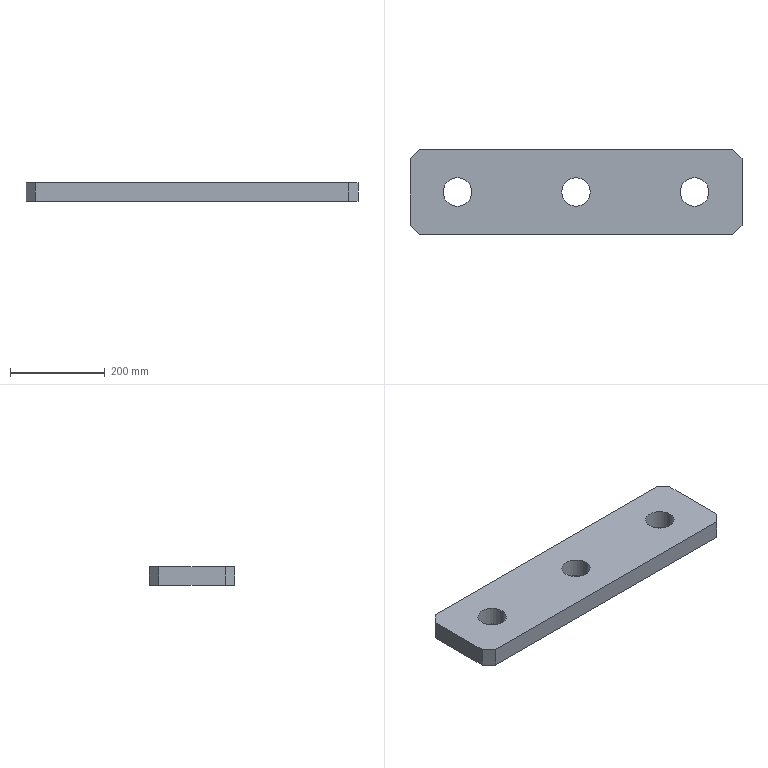Part | STEP file | 001-009-Riveting upper base plate | 1 solid | 16 faces | box 700 x 180 x 40 mm | volume 4668708 mm3 | plane 10 | cylinder 6 | commonest cylinder face diameters 60 x6
STEP:
#1=CARTESIAN_POINT('',(0.,0.,0.));
#2=DIRECTION('',(0.,0.,1.));
#3=DIRECTION('',(1.,0.,0.));
#4=AXIS2_PLACEMENT_3D('',#1,#2,#3);
#5=CARTESIAN_POINT('',(30.,0.,0.));
#6=VERTEX_POINT('',#5);
#7=CARTESIAN_POINT('',(30.,0.,40.));
#8=VERTEX_POINT('',#7);
#9=CARTESIAN_POINT('',(30.,0.,0.));
#10=DIRECTION('',(0.,0.,1.));
#11=VECTOR('',#10,1.);
#12=LINE('',#9,#11);
#13=CARTESIAN_POINT('',(0.,0.,0.));
#14=DIRECTION('',(0.,0.,1.));
#15=DIRECTION('',(1.,0.,0.));
#16=AXIS2_PLACEMENT_3D('',#13,#14,#15);
#17=CYLINDRICAL_SURFACE('',#16,30.);
#18=CARTESIAN_POINT('',(6.283,0.));
#19=DIRECTION('',(0.,1.));
#20=VECTOR('',#19,1.);
#21=LINE('',#18,#20);
#22=(GEOMETRIC_REPRESENTATION_CONTEXT(2)PARAMETRIC_REPRESENTATION_CONTEXT()REPRESENTATION_CONTEXT('',''));
#23=DEFINITIONAL_REPRESENTATION('',(#21),#22);
#24=PCURVE('',#17,#23);
#25=CARTESIAN_POINT('',(0.,0.,0.));
#26=DIRECTION('',(0.,0.,1.));
#27=DIRECTION('',(1.,0.,0.));
#28=AXIS2_PLACEMENT_3D('',#25,#26,#27);
#29=CYLINDRICAL_SURFACE('',#28,30.);
#30=CARTESIAN_POINT('',(0.,0.));
#31=DIRECTION('',(0.,1.));
#32=VECTOR('',#31,1.);
#33=LINE('',#30,#32);
#34=(GEOMETRIC_REPRESENTATION_CONTEXT(2)PARAMETRIC_REPRESENTATION_CONTEXT()REPRESENTATION_CONTEXT('',''));
#35=DEFINITIONAL_REPRESENTATION('',(#33),#34);
#36=PCURVE('',#29,#35);
#37=SURFACE_CURVE('',#12,(#24,#36),.PCURVE_S1.);
#38=EDGE_CURVE('',#6,#8,#37,.T.);
#39=ORIENTED_EDGE('',*,*,#38,.T.);
#40=CARTESIAN_POINT('',(-30.,0.,40.));
#41=VERTEX_POINT('',#40);
#42=CARTESIAN_POINT('',(0.,0.,40.));
#43=DIRECTION('',(0.,0.,1.));
#44=DIRECTION('',(1.,0.,0.));
#45=AXIS2_PLACEMENT_3D('',#42,#43,#44);
#46=CIRCLE('',#45,30.);
#47=CARTESIAN_POINT('',(0.,40.));
#48=DIRECTION('',(1.,0.));
#49=VECTOR('',#48,1.);
#50=LINE('',#47,#49);
#51=(GEOMETRIC_REPRESENTATION_CONTEXT(2)PARAMETRIC_REPRESENTATION_CONTEXT()REPRESENTATION_CONTEXT('',''));
#52=DEFINITIONAL_REPRESENTATION('',(#50),#51);
#53=PCURVE('',#17,#52);
#54=CARTESIAN_POINT('',(0.,0.,40.));
#55=DIRECTION('',(0.,0.,-1.));
#56=DIRECTION('',(-1.,0.,0.));
#57=AXIS2_PLACEMENT_3D('',#54,#55,#56);
#58=PLANE('',#57);
#59=CARTESIAN_POINT('',(-30.,0.));
#60=CARTESIAN_POINT('',(-30.,51.962));
#61=CARTESIAN_POINT('',(15.,25.981));
#62=CARTESIAN_POINT('',(60.,0.));
#63=CARTESIAN_POINT('',(15.,-25.981));
#64=CARTESIAN_POINT('',(-30.,-51.962));
#65=CARTESIAN_POINT('',(-30.,0.));
#66=(BOUNDED_CURVE()B_SPLINE_CURVE(2,(#59,#60,#61,#62,#63,#64,#65),.UNSPECIFIED.,.T.,.F.)B_SPLINE_CURVE_WITH_KNOTS((1,2,2,2,2,1),(-2.094,0.,2.094,4.189,6.283,8.378),.UNSPECIFIED.)CURVE()GEOMETRIC_REPRESENTATION_ITEM()RATIONAL_B_SPLINE_CURVE((1.,0.5,1.,0.5,1.,0.5,1.))REPRESENTATION_ITEM(''));
#67=(GEOMETRIC_REPRESENTATION_CONTEXT(2)PARAMETRIC_REPRESENTATION_CONTEXT()REPRESENTATION_CONTEXT('',''));
#68=DEFINITIONAL_REPRESENTATION('',(#66),#67);
#69=PCURVE('',#58,#68);
#70=SURFACE_CURVE('',#46,(#53,#69),.PCURVE_S1.);
#71=EDGE_CURVE('',#41,#8,#70,.T.);
#72=ORIENTED_EDGE('',*,*,#71,.F.);
#73=CARTESIAN_POINT('',(-30.,0.,0.));
#74=VERTEX_POINT('',#73);
#75=CARTESIAN_POINT('',(-30.,0.,0.));
#76=DIRECTION('',(0.,0.,1.));
#77=VECTOR('',#76,1.);
#78=LINE('',#75,#77);
#79=CARTESIAN_POINT('',(3.142,0.));
#80=DIRECTION('',(0.,1.));
#81=VECTOR('',#80,1.);
#82=LINE('',#79,#81);
#83=(GEOMETRIC_REPRESENTATION_CONTEXT(2)PARAMETRIC_REPRESENTATION_CONTEXT()REPRESENTATION_CONTEXT('',''));
#84=DEFINITIONAL_REPRESENTATION('',(#82),#83);
#85=PCURVE('',#17,#84);
#86=CARTESIAN_POINT('',(3.142,0.));
#87=DIRECTION('',(0.,1.));
#88=VECTOR('',#87,1.);
#89=LINE('',#86,#88);
#90=(GEOMETRIC_REPRESENTATION_CONTEXT(2)PARAMETRIC_REPRESENTATION_CONTEXT()REPRESENTATION_CONTEXT('',''));
#91=DEFINITIONAL_REPRESENTATION('',(#89),#90);
#92=PCURVE('',#29,#91);
#93=SURFACE_CURVE('',#78,(#85,#92),.PCURVE_S1.);
#94=EDGE_CURVE('',#74,#41,#93,.T.);
#95=ORIENTED_EDGE('',*,*,#94,.F.);
#96=CARTESIAN_POINT('',(0.,0.,0.));
#97=DIRECTION('',(0.,0.,1.));
#98=DIRECTION('',(1.,0.,0.));
#99=AXIS2_PLACEMENT_3D('',#96,#97,#98);
#100=CIRCLE('',#99,30.);
#101=CARTESIAN_POINT('',(0.,0.));
#102=DIRECTION('',(1.,0.));
#103=VECTOR('',#102,1.);
#104=LINE('',#101,#103);
#105=(GEOMETRIC_REPRESENTATION_CONTEXT(2)PARAMETRIC_REPRESENTATION_CONTEXT()REPRESENTATION_CONTEXT('',''));
#106=DEFINITIONAL_REPRESENTATION('',(#104),#105);
#107=PCURVE('',#17,#106);
#108=CARTESIAN_POINT('',(0.,0.,0.));
#109=DIRECTION('',(0.,0.,-1.));
#110=DIRECTION('',(-1.,0.,0.));
#111=AXIS2_PLACEMENT_3D('',#108,#109,#110);
#112=PLANE('',#111);
#113=CARTESIAN_POINT('',(-30.,0.));
#114=CARTESIAN_POINT('',(-30.,51.962));
#115=CARTESIAN_POINT('',(15.,25.981));
#116=CARTESIAN_POINT('',(60.,0.));
#117=CARTESIAN_POINT('',(15.,-25.981));
#118=CARTESIAN_POINT('',(-30.,-51.962));
#119=CARTESIAN_POINT('',(-30.,0.));
#120=(BOUNDED_CURVE()B_SPLINE_CURVE(2,(#113,#114,#115,#116,#117,#118,#119),.UNSPECIFIED.,.T.,.F.)B_SPLINE_CURVE_WITH_KNOTS((1,2,2,2,2,1),(-2.094,0.,2.094,4.189,6.283,8.378),.UNSPECIFIED.)CURVE()GEOMETRIC_REPRESENTATION_ITEM()RATIONAL_B_SPLINE_CURVE((1.,0.5,1.,0.5,1.,0.5,1.))REPRESENTATION_ITEM(''));
#121=(GEOMETRIC_REPRESENTATION_CONTEXT(2)PARAMETRIC_REPRESENTATION_CONTEXT()REPRESENTATION_CONTEXT('',''));
#122=DEFINITIONAL_REPRESENTATION('',(#120),#121);
#123=PCURVE('',#112,#122);
#124=SURFACE_CURVE('',#100,(#107,#123),.PCURVE_S1.);
#125=EDGE_CURVE('',#74,#6,#124,.T.);
#126=ORIENTED_EDGE('',*,*,#125,.T.);
#127=EDGE_LOOP('',(#39,#72,#95,#126));
#128=FACE_BOUND('',#127,.F.);
#129=ADVANCED_FACE('',(#128),#17,.F.);
#130=CARTESIAN_POINT('',(220.,0.,40.));
#131=VERTEX_POINT('',#130);
#132=CARTESIAN_POINT('',(220.,0.,0.));
#133=VERTEX_POINT('',#132);
#134=CARTESIAN_POINT('',(220.,0.,40.));
#135=DIRECTION('',(0.,0.,-1.));
#136=VECTOR('',#135,1.);
#137=LINE('',#134,#136);
#138=CARTESIAN_POINT('',(250.,0.,40.));
#139=DIRECTION('',(0.,0.,-1.));
#140=DIRECTION('',(-1.,0.,0.));
#141=AXIS2_PLACEMENT_3D('',#138,#139,#140);
#142=CYLINDRICAL_SURFACE('',#141,30.);
#143=CARTESIAN_POINT('',(6.283,0.));
#144=DIRECTION('',(0.,1.));
#145=VECTOR('',#144,1.);
#146=LINE('',#143,#145);
#147=(GEOMETRIC_REPRESENTATION_CONTEXT(2)PARAMETRIC_REPRESENTATION_CONTEXT()REPRESENTATION_CONTEXT('',''));
#148=DEFINITIONAL_REPRESENTATION('',(#146),#147);
#149=PCURVE('',#142,#148);
#150=CARTESIAN_POINT('',(250.,0.,40.));
#151=DIRECTION('',(0.,0.,-1.));
#152=DIRECTION('',(-1.,0.,0.));
#153=AXIS2_PLACEMENT_3D('',#150,#151,#152);
#154=CYLINDRICAL_SURFACE('',#153,30.);
#155=CARTESIAN_POINT('',(0.,0.));
#156=DIRECTION('',(0.,1.));
#157=VECTOR('',#156,1.);
#158=LINE('',#155,#157);
#159=(GEOMETRIC_REPRESENTATION_CONTEXT(2)PARAMETRIC_REPRESENTATION_CONTEXT()REPRESENTATION_CONTEXT('',''));
#160=DEFINITIONAL_REPRESENTATION('',(#158),#159);
#161=PCURVE('',#154,#160);
#162=SURFACE_CURVE('',#137,(#149,#161),.PCURVE_S1.);
#163=EDGE_CURVE('',#131,#133,#162,.T.);
#164=ORIENTED_EDGE('',*,*,#163,.T.);
#165=CARTESIAN_POINT('',(280.,0.,0.));
#166=VERTEX_POINT('',#165);
#167=CARTESIAN_POINT('',(250.,0.,0.));
#168=DIRECTION('',(0.,0.,-1.));
#169=DIRECTION('',(-1.,0.,0.));
#170=AXIS2_PLACEMENT_3D('',#167,#168,#169);
#171=CIRCLE('',#170,30.);
#172=CARTESIAN_POINT('',(0.,40.));
#173=DIRECTION('',(1.,0.));
#174=VECTOR('',#173,1.);
#175=LINE('',#172,#174);
#176=(GEOMETRIC_REPRESENTATION_CONTEXT(2)PARAMETRIC_REPRESENTATION_CONTEXT()REPRESENTATION_CONTEXT('',''));
#177=DEFINITIONAL_REPRESENTATION('',(#175),#176);
#178=PCURVE('',#142,#177);
#179=CARTESIAN_POINT('',(-250.,0.));
#180=DIRECTION('',(1.,0.));
#181=AXIS2_PLACEMENT_2D('',#179,#180);
#182=CIRCLE('',#181,30.);
#183=(GEOMETRIC_REPRESENTATION_CONTEXT(2)PARAMETRIC_REPRESENTATION_CONTEXT()REPRESENTATION_CONTEXT('',''));
#184=DEFINITIONAL_REPRESENTATION('',(#182),#183);
#185=PCURVE('',#112,#184);
#186=SURFACE_CURVE('',#171,(#178,#185),.PCURVE_S1.);
#187=EDGE_CURVE('',#166,#133,#186,.T.);
#188=ORIENTED_EDGE('',*,*,#187,.F.);
#189=CARTESIAN_POINT('',(280.,0.,40.));
#190=VERTEX_POINT('',#189);
#191=CARTESIAN_POINT('',(280.,0.,40.));
#192=DIRECTION('',(0.,0.,-1.));
#193=VECTOR('',#192,1.);
#194=LINE('',#191,#193);
#195=CARTESIAN_POINT('',(3.142,0.));
#196=DIRECTION('',(0.,1.));
#197=VECTOR('',#196,1.);
#198=LINE('',#195,#197);
#199=(GEOMETRIC_REPRESENTATION_CONTEXT(2)PARAMETRIC_REPRESENTATION_CONTEXT()REPRESENTATION_CONTEXT('',''));
#200=DEFINITIONAL_REPRESENTATION('',(#198),#199);
#201=PCURVE('',#142,#200);
#202=CARTESIAN_POINT('',(3.142,0.));
#203=DIRECTION('',(0.,1.));
#204=VECTOR('',#203,1.);
#205=LINE('',#202,#204);
#206=(GEOMETRIC_REPRESENTATION_CONTEXT(2)PARAMETRIC_REPRESENTATION_CONTEXT()REPRESENTATION_CONTEXT('',''));
#207=DEFINITIONAL_REPRESENTATION('',(#205),#206);
#208=PCURVE('',#154,#207);
#209=SURFACE_CURVE('',#194,(#201,#208),.PCURVE_S1.);
#210=EDGE_CURVE('',#190,#166,#209,.T.);
#211=ORIENTED_EDGE('',*,*,#210,.F.);
#212=CARTESIAN_POINT('',(250.,0.,40.));
#213=DIRECTION('',(0.,0.,-1.));
#214=DIRECTION('',(-1.,0.,0.));
#215=AXIS2_PLACEMENT_3D('',#212,#213,#214);
#216=CIRCLE('',#215,30.);
#217=CARTESIAN_POINT('',(0.,0.));
#218=DIRECTION('',(1.,0.));
#219=VECTOR('',#218,1.);
#220=LINE('',#217,#219);
#221=(GEOMETRIC_REPRESENTATION_CONTEXT(2)PARAMETRIC_REPRESENTATION_CONTEXT()REPRESENTATION_CONTEXT('',''));
#222=DEFINITIONAL_REPRESENTATION('',(#220),#221);
#223=PCURVE('',#142,#222);
#224=CARTESIAN_POINT('',(-250.,0.));
#225=DIRECTION('',(1.,0.));
#226=AXIS2_PLACEMENT_2D('',#224,#225);
#227=CIRCLE('',#226,30.);
#228=(GEOMETRIC_REPRESENTATION_CONTEXT(2)PARAMETRIC_REPRESENTATION_CONTEXT()REPRESENTATION_CONTEXT('',''));
#229=DEFINITIONAL_REPRESENTATION('',(#227),#228);
#230=PCURVE('',#58,#229);
#231=SURFACE_CURVE('',#216,(#223,#230),.PCURVE_S1.);
#232=EDGE_CURVE('',#190,#131,#231,.T.);
#233=ORIENTED_EDGE('',*,*,#232,.T.);
#234=EDGE_LOOP('',(#164,#188,#211,#233));
#235=FACE_BOUND('',#234,.F.);
#236=ADVANCED_FACE('',(#235),#142,.F.);
#237=CARTESIAN_POINT('',(-280.,0.,40.));
#238=VERTEX_POINT('',#237);
#239=CARTESIAN_POINT('',(-280.,0.,0.));
#240=VERTEX_POINT('',#239);
#241=CARTESIAN_POINT('',(-280.,0.,40.));
#242=DIRECTION('',(0.,0.,-1.));
#243=VECTOR('',#242,1.);
#244=LINE('',#241,#243);
#245=CARTESIAN_POINT('',(-250.,0.,40.));
#246=DIRECTION('',(0.,0.,-1.));
#247=DIRECTION('',(-1.,0.,0.));
#248=AXIS2_PLACEMENT_3D('',#245,#246,#247);
#249=CYLINDRICAL_SURFACE('',#248,30.);
#250=CARTESIAN_POINT('',(6.283,0.));
#251=DIRECTION('',(0.,1.));
#252=VECTOR('',#251,1.);
#253=LINE('',#250,#252);
#254=(GEOMETRIC_REPRESENTATION_CONTEXT(2)PARAMETRIC_REPRESENTATION_CONTEXT()REPRESENTATION_CONTEXT('',''));
#255=DEFINITIONAL_REPRESENTATION('',(#253),#254);
#256=PCURVE('',#249,#255);
#257=CARTESIAN_POINT('',(-250.,0.,40.));
#258=DIRECTION('',(0.,0.,-1.));
#259=DIRECTION('',(-1.,0.,0.));
#260=AXIS2_PLACEMENT_3D('',#257,#258,#259);
#261=CYLINDRICAL_SURFACE('',#260,30.);
#262=CARTESIAN_POINT('',(0.,0.));
#263=DIRECTION('',(0.,1.));
#264=VECTOR('',#263,1.);
#265=LINE('',#262,#264);
#266=(GEOMETRIC_REPRESENTATION_CONTEXT(2)PARAMETRIC_REPRESENTATION_CONTEXT()REPRESENTATION_CONTEXT('',''));
#267=DEFINITIONAL_REPRESENTATION('',(#265),#266);
#268=PCURVE('',#261,#267);
#269=SURFACE_CURVE('',#244,(#256,#268),.PCURVE_S1.);
#270=EDGE_CURVE('',#238,#240,#269,.T.);
#271=ORIENTED_EDGE('',*,*,#270,.T.);
#272=CARTESIAN_POINT('',(-220.,0.,0.));
#273=VERTEX_POINT('',#272);
#274=CARTESIAN_POINT('',(-250.,0.,0.));
#275=DIRECTION('',(0.,0.,-1.));
#276=DIRECTION('',(1.,0.,0.));
#277=AXIS2_PLACEMENT_3D('',#274,#275,#276);
#278=CIRCLE('',#277,30.);
#279=CARTESIAN_POINT('',(3.142,40.));
#280=DIRECTION('',(1.,0.));
#281=VECTOR('',#280,1.);
#282=LINE('',#279,#281);
#283=(GEOMETRIC_REPRESENTATION_CONTEXT(2)PARAMETRIC_REPRESENTATION_CONTEXT()REPRESENTATION_CONTEXT('',''));
#284=DEFINITIONAL_REPRESENTATION('',(#282),#283);
#285=PCURVE('',#249,#284);
#286=CARTESIAN_POINT('',(250.,0.));
#287=DIRECTION('',(-1.,0.));
#288=AXIS2_PLACEMENT_2D('',#286,#287);
#289=CIRCLE('',#288,30.);
#290=(GEOMETRIC_REPRESENTATION_CONTEXT(2)PARAMETRIC_REPRESENTATION_CONTEXT()REPRESENTATION_CONTEXT('',''));
#291=DEFINITIONAL_REPRESENTATION('',(#289),#290);
#292=PCURVE('',#112,#291);
#293=SURFACE_CURVE('',#278,(#285,#292),.PCURVE_S1.);
#294=EDGE_CURVE('',#273,#240,#293,.T.);
#295=ORIENTED_EDGE('',*,*,#294,.F.);
#296=CARTESIAN_POINT('',(-220.,0.,40.));
#297=VERTEX_POINT('',#296);
#298=CARTESIAN_POINT('',(-220.,0.,40.));
#299=DIRECTION('',(0.,0.,-1.));
#300=VECTOR('',#299,1.);
#301=LINE('',#298,#300);
#302=CARTESIAN_POINT('',(3.142,0.));
#303=DIRECTION('',(0.,1.));
#304=VECTOR('',#303,1.);
#305=LINE('',#302,#304);
#306=(GEOMETRIC_REPRESENTATION_CONTEXT(2)PARAMETRIC_REPRESENTATION_CONTEXT()REPRESENTATION_CONTEXT('',''));
#307=DEFINITIONAL_REPRESENTATION('',(#305),#306);
#308=PCURVE('',#249,#307);
#309=CARTESIAN_POINT('',(3.142,0.));
#310=DIRECTION('',(0.,1.));
#311=VECTOR('',#310,1.);
#312=LINE('',#309,#311);
#313=(GEOMETRIC_REPRESENTATION_CONTEXT(2)PARAMETRIC_REPRESENTATION_CONTEXT()REPRESENTATION_CONTEXT('',''));
#314=DEFINITIONAL_REPRESENTATION('',(#312),#313);
#315=PCURVE('',#261,#314);
#316=SURFACE_CURVE('',#301,(#308,#315),.PCURVE_S1.);
#317=EDGE_CURVE('',#297,#273,#316,.T.);
#318=ORIENTED_EDGE('',*,*,#317,.F.);
#319=CARTESIAN_POINT('',(-250.,0.,40.));
#320=DIRECTION('',(0.,0.,-1.));
#321=DIRECTION('',(1.,0.,0.));
#322=AXIS2_PLACEMENT_3D('',#319,#320,#321);
#323=CIRCLE('',#322,30.);
#324=CARTESIAN_POINT('',(3.142,0.));
#325=DIRECTION('',(1.,0.));
#326=VECTOR('',#325,1.);
#327=LINE('',#324,#326);
#328=(GEOMETRIC_REPRESENTATION_CONTEXT(2)PARAMETRIC_REPRESENTATION_CONTEXT()REPRESENTATION_CONTEXT('',''));
#329=DEFINITIONAL_REPRESENTATION('',(#327),#328);
#330=PCURVE('',#249,#329);
#331=CARTESIAN_POINT('',(250.,0.));
#332=DIRECTION('',(-1.,0.));
#333=AXIS2_PLACEMENT_2D('',#331,#332);
#334=CIRCLE('',#333,30.);
#335=(GEOMETRIC_REPRESENTATION_CONTEXT(2)PARAMETRIC_REPRESENTATION_CONTEXT()REPRESENTATION_CONTEXT('',''));
#336=DEFINITIONAL_REPRESENTATION('',(#334),#335);
#337=PCURVE('',#58,#336);
#338=SURFACE_CURVE('',#323,(#330,#337),.PCURVE_S1.);
#339=EDGE_CURVE('',#297,#238,#338,.T.);
#340=ORIENTED_EDGE('',*,*,#339,.T.);
#341=EDGE_LOOP('',(#271,#295,#318,#340));
#342=FACE_BOUND('',#341,.F.);
#343=ADVANCED_FACE('',(#342),#249,.F.);
#344=CARTESIAN_POINT('',(350.,-70.,40.));
#345=VERTEX_POINT('',#344);
#346=CARTESIAN_POINT('',(350.,70.,40.));
#347=VERTEX_POINT('',#346);
#348=CARTESIAN_POINT('',(350.,-90.,40.));
#349=DIRECTION('',(0.,1.,0.));
#350=VECTOR('',#349,1.);
#351=LINE('',#348,#350);
#352=CARTESIAN_POINT('',(350.,-90.,40.));
#353=DIRECTION('',(-1.,0.,0.));
#354=DIRECTION('',(0.,0.,1.));
#355=AXIS2_PLACEMENT_3D('',#352,#353,#354);
#356=PLANE('',#355);
#357=CARTESIAN_POINT('',(0.,0.));
#358=DIRECTION('',(0.,1.));
#359=VECTOR('',#358,1.);
#360=LINE('',#357,#359);
#361=(GEOMETRIC_REPRESENTATION_CONTEXT(2)PARAMETRIC_REPRESENTATION_CONTEXT()REPRESENTATION_CONTEXT('',''));
#362=DEFINITIONAL_REPRESENTATION('',(#360),#361);
#363=PCURVE('',#356,#362);
#364=CARTESIAN_POINT('',(-350.,-90.));
#365=DIRECTION('',(0.,1.));
#366=VECTOR('',#365,1.);
#367=LINE('',#364,#366);
#368=(GEOMETRIC_REPRESENTATION_CONTEXT(2)PARAMETRIC_REPRESENTATION_CONTEXT()REPRESENTATION_CONTEXT('',''));
#369=DEFINITIONAL_REPRESENTATION('',(#367),#368);
#370=PCURVE('',#58,#369);
#371=SURFACE_CURVE('',#351,(#363,#370),.PCURVE_S1.);
#372=EDGE_CURVE('',#345,#347,#371,.T.);
#373=ORIENTED_EDGE('',*,*,#372,.F.);
#374=CARTESIAN_POINT('',(350.,-70.,0.));
#375=VERTEX_POINT('',#374);
#376=CARTESIAN_POINT('',(350.,-70.,40.));
#377=DIRECTION('',(0.,0.,-1.));
#378=VECTOR('',#377,1.);
#379=LINE('',#376,#378);
#380=CARTESIAN_POINT('',(0.,20.));
#381=DIRECTION('',(-1.,0.));
#382=VECTOR('',#381,1.);
#383=LINE('',#380,#382);
#384=(GEOMETRIC_REPRESENTATION_CONTEXT(2)PARAMETRIC_REPRESENTATION_CONTEXT()REPRESENTATION_CONTEXT('',''));
#385=DEFINITIONAL_REPRESENTATION('',(#383),#384);
#386=PCURVE('',#356,#385);
#387=CARTESIAN_POINT('',(350.,-70.,40.));
#388=DIRECTION('',(-0.7071,0.7071,0.));
#389=DIRECTION('',(0.,0.,-1.));
#390=AXIS2_PLACEMENT_3D('',#387,#388,#389);
#391=PLANE('',#390);
#392=CARTESIAN_POINT('',(0.,0.));
#393=DIRECTION('',(1.,0.));
#394=VECTOR('',#393,1.);
#395=LINE('',#392,#394);
#396=(GEOMETRIC_REPRESENTATION_CONTEXT(2)PARAMETRIC_REPRESENTATION_CONTEXT()REPRESENTATION_CONTEXT('',''));
#397=DEFINITIONAL_REPRESENTATION('',(#395),#396);
#398=PCURVE('',#391,#397);
#399=SURFACE_CURVE('',#379,(#386,#398),.PCURVE_S1.);
#400=EDGE_CURVE('',#345,#375,#399,.T.);
#401=ORIENTED_EDGE('',*,*,#400,.T.);
#402=CARTESIAN_POINT('',(350.,70.,0.));
#403=VERTEX_POINT('',#402);
#404=CARTESIAN_POINT('',(350.,-90.,0.));
#405=DIRECTION('',(0.,1.,0.));
#406=VECTOR('',#405,1.);
#407=LINE('',#404,#406);
#408=CARTESIAN_POINT('',(-40.,0.));
#409=DIRECTION('',(0.,1.));
#410=VECTOR('',#409,1.);
#411=LINE('',#408,#410);
#412=(GEOMETRIC_REPRESENTATION_CONTEXT(2)PARAMETRIC_REPRESENTATION_CONTEXT()REPRESENTATION_CONTEXT('',''));
#413=DEFINITIONAL_REPRESENTATION('',(#411),#412);
#414=PCURVE('',#356,#413);
#415=CARTESIAN_POINT('',(-350.,-90.));
#416=DIRECTION('',(0.,1.));
#417=VECTOR('',#416,1.);
#418=LINE('',#415,#417);
#419=(GEOMETRIC_REPRESENTATION_CONTEXT(2)PARAMETRIC_REPRESENTATION_CONTEXT()REPRESENTATION_CONTEXT('',''));
#420=DEFINITIONAL_REPRESENTATION('',(#418),#419);
#421=PCURVE('',#112,#420);
#422=SURFACE_CURVE('',#407,(#414,#421),.PCURVE_S1.);
#423=EDGE_CURVE('',#375,#403,#422,.T.);
#424=ORIENTED_EDGE('',*,*,#423,.T.);
#425=CARTESIAN_POINT('',(350.,70.,40.));
#426=DIRECTION('',(0.,0.,1.));
#427=VECTOR('',#426,1.);
#428=LINE('',#425,#427);
#429=CARTESIAN_POINT('',(0.,160.));
#430=DIRECTION('',(1.,0.));
#431=VECTOR('',#430,1.);
#432=LINE('',#429,#431);
#433=(GEOMETRIC_REPRESENTATION_CONTEXT(2)PARAMETRIC_REPRESENTATION_CONTEXT()REPRESENTATION_CONTEXT('',''));
#434=DEFINITIONAL_REPRESENTATION('',(#432),#433);
#435=PCURVE('',#356,#434);
#436=CARTESIAN_POINT('',(330.,90.,40.));
#437=DIRECTION('',(-0.7071,-0.7071,0.));
#438=DIRECTION('',(0.,0.,-1.));
#439=AXIS2_PLACEMENT_3D('',#436,#437,#438);
#440=PLANE('',#439);
#441=CARTESIAN_POINT('',(0.,28.284));
#442=DIRECTION('',(-1.,0.));
#443=VECTOR('',#442,1.);
#444=LINE('',#441,#443);
#445=(GEOMETRIC_REPRESENTATION_CONTEXT(2)PARAMETRIC_REPRESENTATION_CONTEXT()REPRESENTATION_CONTEXT('',''));
#446=DEFINITIONAL_REPRESENTATION('',(#444),#445);
#447=PCURVE('',#440,#446);
#448=SURFACE_CURVE('',#428,(#435,#447),.PCURVE_S1.);
#449=EDGE_CURVE('',#403,#347,#448,.T.);
#450=ORIENTED_EDGE('',*,*,#449,.T.);
#451=EDGE_LOOP('',(#373,#401,#424,#450));
#452=FACE_BOUND('',#451,.T.);
#453=ADVANCED_FACE('',(#452),#356,.F.);
#454=CARTESIAN_POINT('',(330.,90.,40.));
#455=VERTEX_POINT('',#454);
#456=CARTESIAN_POINT('',(-330.,90.,40.));
#457=VERTEX_POINT('',#456);
#458=CARTESIAN_POINT('',(-350.,90.,40.));
#459=DIRECTION('',(-1.,0.,0.));
#460=VECTOR('',#459,1.);
#461=LINE('',#458,#460);
#462=CARTESIAN_POINT('',(-350.,90.,40.));
#463=DIRECTION('',(0.,-1.,0.));
#464=DIRECTION('',(1.,0.,0.));
#465=AXIS2_PLACEMENT_3D('',#462,#463,#464);
#466=PLANE('',#465);
#467=CARTESIAN_POINT('',(0.,0.));
#468=DIRECTION('',(-1.,0.));
#469=VECTOR('',#468,1.);
#470=LINE('',#467,#469);
#471=(GEOMETRIC_REPRESENTATION_CONTEXT(2)PARAMETRIC_REPRESENTATION_CONTEXT()REPRESENTATION_CONTEXT('',''));
#472=DEFINITIONAL_REPRESENTATION('',(#470),#471);
#473=PCURVE('',#466,#472);
#474=CARTESIAN_POINT('',(350.,90.));
#475=DIRECTION('',(1.,0.));
#476=VECTOR('',#475,1.);
#477=LINE('',#474,#476);
#478=(GEOMETRIC_REPRESENTATION_CONTEXT(2)PARAMETRIC_REPRESENTATION_CONTEXT()REPRESENTATION_CONTEXT('',''));
#479=DEFINITIONAL_REPRESENTATION('',(#477),#478);
#480=PCURVE('',#58,#479);
#481=SURFACE_CURVE('',#461,(#473,#480),.PCURVE_S1.);
#482=EDGE_CURVE('',#455,#457,#481,.T.);
#483=ORIENTED_EDGE('',*,*,#482,.F.);
#484=CARTESIAN_POINT('',(330.,90.,0.));
#485=VERTEX_POINT('',#484);
#486=CARTESIAN_POINT('',(330.,90.,40.));
#487=DIRECTION('',(0.,0.,-1.));
#488=VECTOR('',#487,1.);
#489=LINE('',#486,#488);
#490=CARTESIAN_POINT('',(680.,0.));
#491=DIRECTION('',(0.,-1.));
#492=VECTOR('',#491,1.);
#493=LINE('',#490,#492);
#494=(GEOMETRIC_REPRESENTATION_CONTEXT(2)PARAMETRIC_REPRESENTATION_CONTEXT()REPRESENTATION_CONTEXT('',''));
#495=DEFINITIONAL_REPRESENTATION('',(#493),#494);
#496=PCURVE('',#466,#495);
#497=CARTESIAN_POINT('',(0.,0.));
#498=DIRECTION('',(1.,0.));
#499=VECTOR('',#498,1.);
#500=LINE('',#497,#499);
#501=(GEOMETRIC_REPRESENTATION_CONTEXT(2)PARAMETRIC_REPRESENTATION_CONTEXT()REPRESENTATION_CONTEXT('',''));
#502=DEFINITIONAL_REPRESENTATION('',(#500),#501);
#503=PCURVE('',#440,#502);
#504=SURFACE_CURVE('',#489,(#496,#503),.PCURVE_S1.);
#505=EDGE_CURVE('',#455,#485,#504,.T.);
#506=ORIENTED_EDGE('',*,*,#505,.T.);
#507=CARTESIAN_POINT('',(-330.,90.,0.));
#508=VERTEX_POINT('',#507);
#509=CARTESIAN_POINT('',(-350.,90.,0.));
#510=DIRECTION('',(-1.,0.,0.));
#511=VECTOR('',#510,1.);
#512=LINE('',#509,#511);
#513=CARTESIAN_POINT('',(0.,-40.));
#514=DIRECTION('',(-1.,0.));
#515=VECTOR('',#514,1.);
#516=LINE('',#513,#515);
#517=(GEOMETRIC_REPRESENTATION_CONTEXT(2)PARAMETRIC_REPRESENTATION_CONTEXT()REPRESENTATION_CONTEXT('',''));
#518=DEFINITIONAL_REPRESENTATION('',(#516),#517);
#519=PCURVE('',#466,#518);
#520=CARTESIAN_POINT('',(350.,90.));
#521=DIRECTION('',(1.,0.));
#522=VECTOR('',#521,1.);
#523=LINE('',#520,#522);
#524=(GEOMETRIC_REPRESENTATION_CONTEXT(2)PARAMETRIC_REPRESENTATION_CONTEXT()REPRESENTATION_CONTEXT('',''));
#525=DEFINITIONAL_REPRESENTATION('',(#523),#524);
#526=PCURVE('',#112,#525);
#527=SURFACE_CURVE('',#512,(#519,#526),.PCURVE_S1.);
#528=EDGE_CURVE('',#485,#508,#527,.T.);
#529=ORIENTED_EDGE('',*,*,#528,.T.);
#530=CARTESIAN_POINT('',(-330.,90.,40.));
#531=DIRECTION('',(0.,0.,1.));
#532=VECTOR('',#531,1.);
#533=LINE('',#530,#532);
#534=CARTESIAN_POINT('',(20.,0.));
#535=DIRECTION('',(0.,1.));
#536=VECTOR('',#535,1.);
#537=LINE('',#534,#536);
#538=(GEOMETRIC_REPRESENTATION_CONTEXT(2)PARAMETRIC_REPRESENTATION_CONTEXT()REPRESENTATION_CONTEXT('',''));
#539=DEFINITIONAL_REPRESENTATION('',(#537),#538);
#540=PCURVE('',#466,#539);
#541=CARTESIAN_POINT('',(-350.,70.,40.));
#542=DIRECTION('',(0.7071,-0.7071,0.));
#543=DIRECTION('',(0.,0.,-1.));
#544=AXIS2_PLACEMENT_3D('',#541,#542,#543);
#545=PLANE('',#544);
#546=CARTESIAN_POINT('',(0.,28.284));
#547=DIRECTION('',(-1.,0.));
#548=VECTOR('',#547,1.);
#549=LINE('',#546,#548);
#550=(GEOMETRIC_REPRESENTATION_CONTEXT(2)PARAMETRIC_REPRESENTATION_CONTEXT()REPRESENTATION_CONTEXT('',''));
#551=DEFINITIONAL_REPRESENTATION('',(#549),#550);
#552=PCURVE('',#545,#551);
#553=SURFACE_CURVE('',#533,(#540,#552),.PCURVE_S1.);
#554=EDGE_CURVE('',#508,#457,#553,.T.);
#555=ORIENTED_EDGE('',*,*,#554,.T.);
#556=EDGE_LOOP('',(#483,#506,#529,#555));
#557=FACE_BOUND('',#556,.T.);
#558=ADVANCED_FACE('',(#557),#466,.F.);
#559=CARTESIAN_POINT('',(-350.,70.,0.));
#560=VERTEX_POINT('',#559);
#561=CARTESIAN_POINT('',(-350.,-70.,0.));
#562=VERTEX_POINT('',#561);
#563=CARTESIAN_POINT('',(-350.,-90.,0.));
#564=DIRECTION('',(0.,-1.,0.));
#565=VECTOR('',#564,1.);
#566=LINE('',#563,#565);
#567=CARTESIAN_POINT('',(-350.,-90.,40.));
#568=DIRECTION('',(1.,0.,0.));
#569=DIRECTION('',(0.,1.,0.));
#570=AXIS2_PLACEMENT_3D('',#567,#568,#569);
#571=PLANE('',#570);
#572=CARTESIAN_POINT('',(0.,-40.));
#573=DIRECTION('',(-1.,0.));
#574=VECTOR('',#573,1.);
#575=LINE('',#572,#574);
#576=(GEOMETRIC_REPRESENTATION_CONTEXT(2)PARAMETRIC_REPRESENTATION_CONTEXT()REPRESENTATION_CONTEXT('',''));
#577=DEFINITIONAL_REPRESENTATION('',(#575),#576);
#578=PCURVE('',#571,#577);
#579=CARTESIAN_POINT('',(350.,-90.));
#580=DIRECTION('',(0.,-1.));
#581=VECTOR('',#580,1.);
#582=LINE('',#579,#581);
#583=(GEOMETRIC_REPRESENTATION_CONTEXT(2)PARAMETRIC_REPRESENTATION_CONTEXT()REPRESENTATION_CONTEXT('',''));
#584=DEFINITIONAL_REPRESENTATION('',(#582),#583);
#585=PCURVE('',#112,#584);
#586=SURFACE_CURVE('',#566,(#578,#585),.PCURVE_S1.);
#587=EDGE_CURVE('',#560,#562,#586,.T.);
#588=ORIENTED_EDGE('',*,*,#587,.T.);
#589=CARTESIAN_POINT('',(-350.,-70.,40.));
#590=VERTEX_POINT('',#589);
#591=CARTESIAN_POINT('',(-350.,-70.,40.));
#592=DIRECTION('',(0.,0.,1.));
#593=VECTOR('',#592,1.);
#594=LINE('',#591,#593);
#595=CARTESIAN_POINT('',(20.,0.));
#596=DIRECTION('',(0.,1.));
#597=VECTOR('',#596,1.);
#598=LINE('',#595,#597);
#599=(GEOMETRIC_REPRESENTATION_CONTEXT(2)PARAMETRIC_REPRESENTATION_CONTEXT()REPRESENTATION_CONTEXT('',''));
#600=DEFINITIONAL_REPRESENTATION('',(#598),#599);
#601=PCURVE('',#571,#600);
#602=CARTESIAN_POINT('',(-330.,-90.,40.));
#603=DIRECTION('',(0.7071,0.7071,0.));
#604=DIRECTION('',(0.,0.,-1.));
#605=AXIS2_PLACEMENT_3D('',#602,#603,#604);
#606=PLANE('',#605);
#607=CARTESIAN_POINT('',(0.,28.284));
#608=DIRECTION('',(-1.,0.));
#609=VECTOR('',#608,1.);
#610=LINE('',#607,#609);
#611=(GEOMETRIC_REPRESENTATION_CONTEXT(2)PARAMETRIC_REPRESENTATION_CONTEXT()REPRESENTATION_CONTEXT('',''));
#612=DEFINITIONAL_REPRESENTATION('',(#610),#611);
#613=PCURVE('',#606,#612);
#614=SURFACE_CURVE('',#594,(#601,#613),.PCURVE_S1.);
#615=EDGE_CURVE('',#562,#590,#614,.T.);
#616=ORIENTED_EDGE('',*,*,#615,.T.);
#617=CARTESIAN_POINT('',(-350.,70.,40.));
#618=VERTEX_POINT('',#617);
#619=CARTESIAN_POINT('',(-350.,-90.,40.));
#620=DIRECTION('',(0.,-1.,0.));
#621=VECTOR('',#620,1.);
#622=LINE('',#619,#621);
#623=CARTESIAN_POINT('',(0.,0.));
#624=DIRECTION('',(-1.,0.));
#625=VECTOR('',#624,1.);
#626=LINE('',#623,#625);
#627=(GEOMETRIC_REPRESENTATION_CONTEXT(2)PARAMETRIC_REPRESENTATION_CONTEXT()REPRESENTATION_CONTEXT('',''));
#628=DEFINITIONAL_REPRESENTATION('',(#626),#627);
#629=PCURVE('',#571,#628);
#630=CARTESIAN_POINT('',(350.,-90.));
#631=DIRECTION('',(0.,-1.));
#632=VECTOR('',#631,1.);
#633=LINE('',#630,#632);
#634=(GEOMETRIC_REPRESENTATION_CONTEXT(2)PARAMETRIC_REPRESENTATION_CONTEXT()REPRESENTATION_CONTEXT('',''));
#635=DEFINITIONAL_REPRESENTATION('',(#633),#634);
#636=PCURVE('',#58,#635);
#637=SURFACE_CURVE('',#622,(#629,#636),.PCURVE_S1.);
#638=EDGE_CURVE('',#618,#590,#637,.T.);
#639=ORIENTED_EDGE('',*,*,#638,.F.);
#640=CARTESIAN_POINT('',(-350.,70.,40.));
#641=DIRECTION('',(0.,0.,-1.));
#642=VECTOR('',#641,1.);
#643=LINE('',#640,#642);
#644=CARTESIAN_POINT('',(160.,0.));
#645=DIRECTION('',(0.,-1.));
#646=VECTOR('',#645,1.);
#647=LINE('',#644,#646);
#648=(GEOMETRIC_REPRESENTATION_CONTEXT(2)PARAMETRIC_REPRESENTATION_CONTEXT()REPRESENTATION_CONTEXT('',''));
#649=DEFINITIONAL_REPRESENTATION('',(#647),#648);
#650=PCURVE('',#571,#649);
#651=CARTESIAN_POINT('',(0.,0.));
#652=DIRECTION('',(1.,0.));
#653=VECTOR('',#652,1.);
#654=LINE('',#651,#653);
#655=(GEOMETRIC_REPRESENTATION_CONTEXT(2)PARAMETRIC_REPRESENTATION_CONTEXT()REPRESENTATION_CONTEXT('',''));
#656=DEFINITIONAL_REPRESENTATION('',(#654),#655);
#657=PCURVE('',#545,#656);
#658=SURFACE_CURVE('',#643,(#650,#657),.PCURVE_S1.);
#659=EDGE_CURVE('',#618,#560,#658,.T.);
#660=ORIENTED_EDGE('',*,*,#659,.T.);
#661=EDGE_LOOP('',(#588,#616,#639,#660));
#662=FACE_BOUND('',#661,.T.);
#663=ADVANCED_FACE('',(#662),#571,.F.);
#664=CARTESIAN_POINT('',(-330.,-90.,0.));
#665=VERTEX_POINT('',#664);
#666=CARTESIAN_POINT('',(330.,-90.,0.));
#667=VERTEX_POINT('',#666);
#668=CARTESIAN_POINT('',(-350.,-90.,0.));
#669=DIRECTION('',(1.,0.,0.));
#670=VECTOR('',#669,1.);
#671=LINE('',#668,#670);
#672=CARTESIAN_POINT('',(-350.,-90.,40.));
#673=DIRECTION('',(0.,1.,0.));
#674=DIRECTION('',(-1.,0.,0.));
#675=AXIS2_PLACEMENT_3D('',#672,#673,#674);
#676=PLANE('',#675);
#677=CARTESIAN_POINT('',(0.,-40.));
#678=DIRECTION('',(-1.,0.));
#679=VECTOR('',#678,1.);
#680=LINE('',#677,#679);
#681=(GEOMETRIC_REPRESENTATION_CONTEXT(2)PARAMETRIC_REPRESENTATION_CONTEXT()REPRESENTATION_CONTEXT('',''));
#682=DEFINITIONAL_REPRESENTATION('',(#680),#681);
#683=PCURVE('',#676,#682);
#684=CARTESIAN_POINT('',(350.,-90.));
#685=DIRECTION('',(-1.,0.));
#686=VECTOR('',#685,1.);
#687=LINE('',#684,#686);
#688=(GEOMETRIC_REPRESENTATION_CONTEXT(2)PARAMETRIC_REPRESENTATION_CONTEXT()REPRESENTATION_CONTEXT('',''));
#689=DEFINITIONAL_REPRESENTATION('',(#687),#688);
#690=PCURVE('',#112,#689);
#691=SURFACE_CURVE('',#671,(#683,#690),.PCURVE_S1.);
#692=EDGE_CURVE('',#665,#667,#691,.T.);
#693=ORIENTED_EDGE('',*,*,#692,.T.);
#694=CARTESIAN_POINT('',(330.,-90.,40.));
#695=VERTEX_POINT('',#694);
#696=CARTESIAN_POINT('',(330.,-90.,40.));
#697=DIRECTION('',(0.,0.,1.));
#698=VECTOR('',#697,1.);
#699=LINE('',#696,#698);
#700=CARTESIAN_POINT('',(-680.,0.));
#701=DIRECTION('',(0.,1.));
#702=VECTOR('',#701,1.);
#703=LINE('',#700,#702);
#704=(GEOMETRIC_REPRESENTATION_CONTEXT(2)PARAMETRIC_REPRESENTATION_CONTEXT()REPRESENTATION_CONTEXT('',''));
#705=DEFINITIONAL_REPRESENTATION('',(#703),#704);
#706=PCURVE('',#676,#705);
#707=CARTESIAN_POINT('',(0.,28.284));
#708=DIRECTION('',(-1.,0.));
#709=VECTOR('',#708,1.);
#710=LINE('',#707,#709);
#711=(GEOMETRIC_REPRESENTATION_CONTEXT(2)PARAMETRIC_REPRESENTATION_CONTEXT()REPRESENTATION_CONTEXT('',''));
#712=DEFINITIONAL_REPRESENTATION('',(#710),#711);
#713=PCURVE('',#391,#712);
#714=SURFACE_CURVE('',#699,(#706,#713),.PCURVE_S1.);
#715=EDGE_CURVE('',#667,#695,#714,.T.);
#716=ORIENTED_EDGE('',*,*,#715,.T.);
#717=CARTESIAN_POINT('',(-330.,-90.,40.));
#718=VERTEX_POINT('',#717);
#719=CARTESIAN_POINT('',(-350.,-90.,40.));
#720=DIRECTION('',(1.,0.,0.));
#721=VECTOR('',#720,1.);
#722=LINE('',#719,#721);
#723=CARTESIAN_POINT('',(0.,0.));
#724=DIRECTION('',(-1.,0.));
#725=VECTOR('',#724,1.);
#726=LINE('',#723,#725);
#727=(GEOMETRIC_REPRESENTATION_CONTEXT(2)PARAMETRIC_REPRESENTATION_CONTEXT()REPRESENTATION_CONTEXT('',''));
#728=DEFINITIONAL_REPRESENTATION('',(#726),#727);
#729=PCURVE('',#676,#728);
#730=CARTESIAN_POINT('',(350.,-90.));
#731=DIRECTION('',(-1.,0.));
#732=VECTOR('',#731,1.);
#733=LINE('',#730,#732);
#734=(GEOMETRIC_REPRESENTATION_CONTEXT(2)PARAMETRIC_REPRESENTATION_CONTEXT()REPRESENTATION_CONTEXT('',''));
#735=DEFINITIONAL_REPRESENTATION('',(#733),#734);
#736=PCURVE('',#58,#735);
#737=SURFACE_CURVE('',#722,(#729,#736),.PCURVE_S1.);
#738=EDGE_CURVE('',#718,#695,#737,.T.);
#739=ORIENTED_EDGE('',*,*,#738,.F.);
#740=CARTESIAN_POINT('',(-330.,-90.,40.));
#741=DIRECTION('',(0.,0.,-1.));
#742=VECTOR('',#741,1.);
#743=LINE('',#740,#742);
#744=CARTESIAN_POINT('',(-20.,0.));
#745=DIRECTION('',(0.,-1.));
#746=VECTOR('',#745,1.);
#747=LINE('',#744,#746);
#748=(GEOMETRIC_REPRESENTATION_CONTEXT(2)PARAMETRIC_REPRESENTATION_CONTEXT()REPRESENTATION_CONTEXT('',''));
#749=DEFINITIONAL_REPRESENTATION('',(#747),#748);
#750=PCURVE('',#676,#749);
#751=CARTESIAN_POINT('',(0.,0.));
#752=DIRECTION('',(1.,0.));
#753=VECTOR('',#752,1.);
#754=LINE('',#751,#753);
#755=(GEOMETRIC_REPRESENTATION_CONTEXT(2)PARAMETRIC_REPRESENTATION_CONTEXT()REPRESENTATION_CONTEXT('',''));
#756=DEFINITIONAL_REPRESENTATION('',(#754),#755);
#757=PCURVE('',#606,#756);
#758=SURFACE_CURVE('',#743,(#750,#757),.PCURVE_S1.);
#759=EDGE_CURVE('',#718,#665,#758,.T.);
#760=ORIENTED_EDGE('',*,*,#759,.T.);
#761=EDGE_LOOP('',(#693,#716,#739,#760));
#762=FACE_BOUND('',#761,.T.);
#763=ADVANCED_FACE('',(#762),#676,.F.);
#764=CARTESIAN_POINT('',(0.,0.,40.));
#765=DIRECTION('',(0.,0.,1.));
#766=DIRECTION('',(1.,0.,0.));
#767=AXIS2_PLACEMENT_3D('',#764,#765,#766);
#768=CIRCLE('',#767,30.);
#769=CARTESIAN_POINT('',(-30.,0.));
#770=CARTESIAN_POINT('',(-30.,51.962));
#771=CARTESIAN_POINT('',(15.,25.981));
#772=CARTESIAN_POINT('',(60.,0.));
#773=CARTESIAN_POINT('',(15.,-25.981));
#774=CARTESIAN_POINT('',(-30.,-51.962));
#775=CARTESIAN_POINT('',(-30.,0.));
#776=(BOUNDED_CURVE()B_SPLINE_CURVE(2,(#769,#770,#771,#772,#773,#774,#775),.UNSPECIFIED.,.T.,.F.)B_SPLINE_CURVE_WITH_KNOTS((1,2,2,2,2,1),(-2.094,0.,2.094,4.189,6.283,8.378),.UNSPECIFIED.)CURVE()GEOMETRIC_REPRESENTATION_ITEM()RATIONAL_B_SPLINE_CURVE((1.,0.5,1.,0.5,1.,0.5,1.))REPRESENTATION_ITEM(''));
#777=(GEOMETRIC_REPRESENTATION_CONTEXT(2)PARAMETRIC_REPRESENTATION_CONTEXT()REPRESENTATION_CONTEXT('',''));
#778=DEFINITIONAL_REPRESENTATION('',(#776),#777);
#779=PCURVE('',#58,#778);
#780=CARTESIAN_POINT('',(0.,40.));
#781=DIRECTION('',(1.,0.));
#782=VECTOR('',#781,1.);
#783=LINE('',#780,#782);
#784=(GEOMETRIC_REPRESENTATION_CONTEXT(2)PARAMETRIC_REPRESENTATION_CONTEXT()REPRESENTATION_CONTEXT('',''));
#785=DEFINITIONAL_REPRESENTATION('',(#783),#784);
#786=PCURVE('',#29,#785);
#787=SURFACE_CURVE('',#768,(#779,#786),.PCURVE_S1.);
#788=EDGE_CURVE('',#8,#41,#787,.T.);
#789=ORIENTED_EDGE('',*,*,#788,.F.);
#790=ORIENTED_EDGE('',*,*,#71,.F.);
#791=EDGE_LOOP('',(#789,#790));
#792=FACE_BOUND('',#791,.T.);
#793=CARTESIAN_POINT('',(250.,0.,40.));
#794=DIRECTION('',(0.,0.,-1.));
#795=DIRECTION('',(-1.,0.,0.));
#796=AXIS2_PLACEMENT_3D('',#793,#794,#795);
#797=CIRCLE('',#796,30.);
#798=CARTESIAN_POINT('',(-250.,0.));
#799=DIRECTION('',(1.,0.));
#800=AXIS2_PLACEMENT_2D('',#798,#799);
#801=CIRCLE('',#800,30.);
#802=(GEOMETRIC_REPRESENTATION_CONTEXT(2)PARAMETRIC_REPRESENTATION_CONTEXT()REPRESENTATION_CONTEXT('',''));
#803=DEFINITIONAL_REPRESENTATION('',(#801),#802);
#804=PCURVE('',#58,#803);
#805=CARTESIAN_POINT('',(0.,0.));
#806=DIRECTION('',(1.,0.));
#807=VECTOR('',#806,1.);
#808=LINE('',#805,#807);
#809=(GEOMETRIC_REPRESENTATION_CONTEXT(2)PARAMETRIC_REPRESENTATION_CONTEXT()REPRESENTATION_CONTEXT('',''));
#810=DEFINITIONAL_REPRESENTATION('',(#808),#809);
#811=PCURVE('',#154,#810);
#812=SURFACE_CURVE('',#797,(#804,#811),.PCURVE_S1.);
#813=EDGE_CURVE('',#131,#190,#812,.T.);
#814=ORIENTED_EDGE('',*,*,#813,.T.);
#815=ORIENTED_EDGE('',*,*,#232,.T.);
#816=EDGE_LOOP('',(#814,#815));
#817=FACE_BOUND('',#816,.T.);
#818=CARTESIAN_POINT('',(-250.,0.,40.));
#819=DIRECTION('',(0.,0.,-1.));
#820=DIRECTION('',(1.,0.,0.));
#821=AXIS2_PLACEMENT_3D('',#818,#819,#820);
#822=CIRCLE('',#821,30.);
#823=CARTESIAN_POINT('',(250.,0.));
#824=DIRECTION('',(-1.,0.));
#825=AXIS2_PLACEMENT_2D('',#823,#824);
#826=CIRCLE('',#825,30.);
#827=(GEOMETRIC_REPRESENTATION_CONTEXT(2)PARAMETRIC_REPRESENTATION_CONTEXT()REPRESENTATION_CONTEXT('',''));
#828=DEFINITIONAL_REPRESENTATION('',(#826),#827);
#829=PCURVE('',#58,#828);
#830=CARTESIAN_POINT('',(-3.142,0.));
#831=DIRECTION('',(1.,0.));
#832=VECTOR('',#831,1.);
#833=LINE('',#830,#832);
#834=(GEOMETRIC_REPRESENTATION_CONTEXT(2)PARAMETRIC_REPRESENTATION_CONTEXT()REPRESENTATION_CONTEXT('',''));
#835=DEFINITIONAL_REPRESENTATION('',(#833),#834);
#836=PCURVE('',#261,#835);
#837=SURFACE_CURVE('',#822,(#829,#836),.PCURVE_S1.);
#838=EDGE_CURVE('',#238,#297,#837,.T.);
#839=ORIENTED_EDGE('',*,*,#838,.T.);
#840=ORIENTED_EDGE('',*,*,#339,.T.);
#841=EDGE_LOOP('',(#839,#840));
#842=FACE_BOUND('',#841,.T.);
#843=ORIENTED_EDGE('',*,*,#738,.T.);
#844=CARTESIAN_POINT('',(350.,-70.,40.));
#845=DIRECTION('',(0.7071,0.7071,0.));
#846=VECTOR('',#845,1.);
#847=LINE('',#844,#846);
#848=CARTESIAN_POINT('',(-350.,-70.));
#849=DIRECTION('',(-0.7071,0.7071));
#850=VECTOR('',#849,1.);
#851=LINE('',#848,#850);
#852=(GEOMETRIC_REPRESENTATION_CONTEXT(2)PARAMETRIC_REPRESENTATION_CONTEXT()REPRESENTATION_CONTEXT('',''));
#853=DEFINITIONAL_REPRESENTATION('',(#851),#852);
#854=PCURVE('',#58,#853);
#855=CARTESIAN_POINT('',(0.,0.));
#856=DIRECTION('',(0.,-1.));
#857=VECTOR('',#856,1.);
#858=LINE('',#855,#857);
#859=(GEOMETRIC_REPRESENTATION_CONTEXT(2)PARAMETRIC_REPRESENTATION_CONTEXT()REPRESENTATION_CONTEXT('',''));
#860=DEFINITIONAL_REPRESENTATION('',(#858),#859);
#861=PCURVE('',#391,#860);
#862=SURFACE_CURVE('',#847,(#854,#861),.PCURVE_S1.);
#863=EDGE_CURVE('',#695,#345,#862,.T.);
#864=ORIENTED_EDGE('',*,*,#863,.T.);
#865=ORIENTED_EDGE('',*,*,#372,.T.);
#866=CARTESIAN_POINT('',(330.,90.,40.));
#867=DIRECTION('',(-0.7071,0.7071,0.));
#868=VECTOR('',#867,1.);
#869=LINE('',#866,#868);
#870=CARTESIAN_POINT('',(-330.,90.));
#871=DIRECTION('',(0.7071,0.7071));
#872=VECTOR('',#871,1.);
#873=LINE('',#870,#872);
#874=(GEOMETRIC_REPRESENTATION_CONTEXT(2)PARAMETRIC_REPRESENTATION_CONTEXT()REPRESENTATION_CONTEXT('',''));
#875=DEFINITIONAL_REPRESENTATION('',(#873),#874);
#876=PCURVE('',#58,#875);
#877=CARTESIAN_POINT('',(0.,0.));
#878=DIRECTION('',(0.,-1.));
#879=VECTOR('',#878,1.);
#880=LINE('',#877,#879);
#881=(GEOMETRIC_REPRESENTATION_CONTEXT(2)PARAMETRIC_REPRESENTATION_CONTEXT()REPRESENTATION_CONTEXT('',''));
#882=DEFINITIONAL_REPRESENTATION('',(#880),#881);
#883=PCURVE('',#440,#882);
#884=SURFACE_CURVE('',#869,(#876,#883),.PCURVE_S1.);
#885=EDGE_CURVE('',#347,#455,#884,.T.);
#886=ORIENTED_EDGE('',*,*,#885,.T.);
#887=ORIENTED_EDGE('',*,*,#482,.T.);
#888=CARTESIAN_POINT('',(-350.,70.,40.));
#889=DIRECTION('',(-0.7071,-0.7071,0.));
#890=VECTOR('',#889,1.);
#891=LINE('',#888,#890);
#892=CARTESIAN_POINT('',(350.,70.));
#893=DIRECTION('',(0.7071,-0.7071));
#894=VECTOR('',#893,1.);
#895=LINE('',#892,#894);
#896=(GEOMETRIC_REPRESENTATION_CONTEXT(2)PARAMETRIC_REPRESENTATION_CONTEXT()REPRESENTATION_CONTEXT('',''));
#897=DEFINITIONAL_REPRESENTATION('',(#895),#896);
#898=PCURVE('',#58,#897);
#899=CARTESIAN_POINT('',(0.,0.));
#900=DIRECTION('',(0.,-1.));
#901=VECTOR('',#900,1.);
#902=LINE('',#899,#901);
#903=(GEOMETRIC_REPRESENTATION_CONTEXT(2)PARAMETRIC_REPRESENTATION_CONTEXT()REPRESENTATION_CONTEXT('',''));
#904=DEFINITIONAL_REPRESENTATION('',(#902),#903);
#905=PCURVE('',#545,#904);
#906=SURFACE_CURVE('',#891,(#898,#905),.PCURVE_S1.);
#907=EDGE_CURVE('',#457,#618,#906,.T.);
#908=ORIENTED_EDGE('',*,*,#907,.T.);
#909=ORIENTED_EDGE('',*,*,#638,.T.);
#910=CARTESIAN_POINT('',(-330.,-90.,40.));
#911=DIRECTION('',(0.7071,-0.7071,0.));
#912=VECTOR('',#911,1.);
#913=LINE('',#910,#912);
#914=CARTESIAN_POINT('',(330.,-90.));
#915=DIRECTION('',(-0.7071,-0.7071));
#916=VECTOR('',#915,1.);
#917=LINE('',#914,#916);
#918=(GEOMETRIC_REPRESENTATION_CONTEXT(2)PARAMETRIC_REPRESENTATION_CONTEXT()REPRESENTATION_CONTEXT('',''));
#919=DEFINITIONAL_REPRESENTATION('',(#917),#918);
#920=PCURVE('',#58,#919);
#921=CARTESIAN_POINT('',(0.,0.));
#922=DIRECTION('',(0.,-1.));
#923=VECTOR('',#922,1.);
#924=LINE('',#921,#923);
#925=(GEOMETRIC_REPRESENTATION_CONTEXT(2)PARAMETRIC_REPRESENTATION_CONTEXT()REPRESENTATION_CONTEXT('',''));
#926=DEFINITIONAL_REPRESENTATION('',(#924),#925);
#927=PCURVE('',#606,#926);
#928=SURFACE_CURVE('',#913,(#920,#927),.PCURVE_S1.);
#929=EDGE_CURVE('',#590,#718,#928,.T.);
#930=ORIENTED_EDGE('',*,*,#929,.T.);
#931=EDGE_LOOP('',(#843,#864,#865,#886,#887,#908,#909,#930));
#932=FACE_BOUND('',#931,.T.);
#933=ADVANCED_FACE('',(#792,#817,#842,#932),#58,.F.);
#934=CARTESIAN_POINT('',(0.,0.,0.));
#935=DIRECTION('',(0.,0.,1.));
#936=DIRECTION('',(1.,0.,0.));
#937=AXIS2_PLACEMENT_3D('',#934,#935,#936);
#938=CIRCLE('',#937,30.);
#939=CARTESIAN_POINT('',(-30.,0.));
#940=CARTESIAN_POINT('',(-30.,51.962));
#941=CARTESIAN_POINT('',(15.,25.981));
#942=CARTESIAN_POINT('',(60.,0.));
#943=CARTESIAN_POINT('',(15.,-25.981));
#944=CARTESIAN_POINT('',(-30.,-51.962));
#945=CARTESIAN_POINT('',(-30.,0.));
#946=(BOUNDED_CURVE()B_SPLINE_CURVE(2,(#939,#940,#941,#942,#943,#944,#945),.UNSPECIFIED.,.T.,.F.)B_SPLINE_CURVE_WITH_KNOTS((1,2,2,2,2,1),(-2.094,0.,2.094,4.189,6.283,8.378),.UNSPECIFIED.)CURVE()GEOMETRIC_REPRESENTATION_ITEM()RATIONAL_B_SPLINE_CURVE((1.,0.5,1.,0.5,1.,0.5,1.))REPRESENTATION_ITEM(''));
#947=(GEOMETRIC_REPRESENTATION_CONTEXT(2)PARAMETRIC_REPRESENTATION_CONTEXT()REPRESENTATION_CONTEXT('',''));
#948=DEFINITIONAL_REPRESENTATION('',(#946),#947);
#949=PCURVE('',#112,#948);
#950=CARTESIAN_POINT('',(0.,0.));
#951=DIRECTION('',(1.,0.));
#952=VECTOR('',#951,1.);
#953=LINE('',#950,#952);
#954=(GEOMETRIC_REPRESENTATION_CONTEXT(2)PARAMETRIC_REPRESENTATION_CONTEXT()REPRESENTATION_CONTEXT('',''));
#955=DEFINITIONAL_REPRESENTATION('',(#953),#954);
#956=PCURVE('',#29,#955);
#957=SURFACE_CURVE('',#938,(#949,#956),.PCURVE_S1.);
#958=EDGE_CURVE('',#6,#74,#957,.T.);
#959=ORIENTED_EDGE('',*,*,#958,.T.);
#960=ORIENTED_EDGE('',*,*,#125,.T.);
#961=EDGE_LOOP('',(#959,#960));
#962=FACE_BOUND('',#961,.T.);
#963=CARTESIAN_POINT('',(250.,0.,0.));
#964=DIRECTION('',(0.,0.,-1.));
#965=DIRECTION('',(-1.,0.,0.));
#966=AXIS2_PLACEMENT_3D('',#963,#964,#965);
#967=CIRCLE('',#966,30.);
#968=CARTESIAN_POINT('',(-250.,0.));
#969=DIRECTION('',(1.,0.));
#970=AXIS2_PLACEMENT_2D('',#968,#969);
#971=CIRCLE('',#970,30.);
#972=(GEOMETRIC_REPRESENTATION_CONTEXT(2)PARAMETRIC_REPRESENTATION_CONTEXT()REPRESENTATION_CONTEXT('',''));
#973=DEFINITIONAL_REPRESENTATION('',(#971),#972);
#974=PCURVE('',#112,#973);
#975=CARTESIAN_POINT('',(0.,40.));
#976=DIRECTION('',(1.,0.));
#977=VECTOR('',#976,1.);
#978=LINE('',#975,#977);
#979=(GEOMETRIC_REPRESENTATION_CONTEXT(2)PARAMETRIC_REPRESENTATION_CONTEXT()REPRESENTATION_CONTEXT('',''));
#980=DEFINITIONAL_REPRESENTATION('',(#978),#979);
#981=PCURVE('',#154,#980);
#982=SURFACE_CURVE('',#967,(#974,#981),.PCURVE_S1.);
#983=EDGE_CURVE('',#133,#166,#982,.T.);
#984=ORIENTED_EDGE('',*,*,#983,.F.);
#985=ORIENTED_EDGE('',*,*,#187,.F.);
#986=EDGE_LOOP('',(#984,#985));
#987=FACE_BOUND('',#986,.T.);
#988=CARTESIAN_POINT('',(-250.,0.,0.));
#989=DIRECTION('',(0.,0.,-1.));
#990=DIRECTION('',(1.,0.,0.));
#991=AXIS2_PLACEMENT_3D('',#988,#989,#990);
#992=CIRCLE('',#991,30.);
#993=CARTESIAN_POINT('',(250.,0.));
#994=DIRECTION('',(-1.,0.));
#995=AXIS2_PLACEMENT_2D('',#993,#994);
#996=CIRCLE('',#995,30.);
#997=(GEOMETRIC_REPRESENTATION_CONTEXT(2)PARAMETRIC_REPRESENTATION_CONTEXT()REPRESENTATION_CONTEXT('',''));
#998=DEFINITIONAL_REPRESENTATION('',(#996),#997);
#999=PCURVE('',#112,#998);
#1000=CARTESIAN_POINT('',(-3.142,40.));
#1001=DIRECTION('',(1.,0.));
#1002=VECTOR('',#1001,1.);
#1003=LINE('',#1000,#1002);
#1004=(GEOMETRIC_REPRESENTATION_CONTEXT(2)PARAMETRIC_REPRESENTATION_CONTEXT()REPRESENTATION_CONTEXT('',''));
#1005=DEFINITIONAL_REPRESENTATION('',(#1003),#1004);
#1006=PCURVE('',#261,#1005);
#1007=SURFACE_CURVE('',#992,(#999,#1006),.PCURVE_S1.);
#1008=EDGE_CURVE('',#240,#273,#1007,.T.);
#1009=ORIENTED_EDGE('',*,*,#1008,.F.);
#1010=ORIENTED_EDGE('',*,*,#294,.F.);
#1011=EDGE_LOOP('',(#1009,#1010));
#1012=FACE_BOUND('',#1011,.T.);
#1013=ORIENTED_EDGE('',*,*,#423,.F.);
#1014=CARTESIAN_POINT('',(210.,-210.,0.));
#1015=DIRECTION('',(-0.7071,-0.7071,0.));
#1016=VECTOR('',#1015,1.);
#1017=LINE('',#1014,#1016);
#1018=CARTESIAN_POINT('',(-210.,-210.));
#1019=DIRECTION('',(0.7071,-0.7071));
#1020=VECTOR('',#1019,1.);
#1021=LINE('',#1018,#1020);
#1022=(GEOMETRIC_REPRESENTATION_CONTEXT(2)PARAMETRIC_REPRESENTATION_CONTEXT()REPRESENTATION_CONTEXT('',''));
#1023=DEFINITIONAL_REPRESENTATION('',(#1021),#1022);
#1024=PCURVE('',#112,#1023);
#1025=CARTESIAN_POINT('',(40.,197.99));
#1026=DIRECTION('',(0.,1.));
#1027=VECTOR('',#1026,1.);
#1028=LINE('',#1025,#1027);
#1029=(GEOMETRIC_REPRESENTATION_CONTEXT(2)PARAMETRIC_REPRESENTATION_CONTEXT()REPRESENTATION_CONTEXT('',''));
#1030=DEFINITIONAL_REPRESENTATION('',(#1028),#1029);
#1031=PCURVE('',#391,#1030);
#1032=SURFACE_CURVE('',#1017,(#1024,#1031),.PCURVE_S1.);
#1033=EDGE_CURVE('',#375,#667,#1032,.T.);
#1034=ORIENTED_EDGE('',*,*,#1033,.T.);
#1035=ORIENTED_EDGE('',*,*,#692,.F.);
#1036=CARTESIAN_POINT('',(-210.,-210.,0.));
#1037=DIRECTION('',(-0.7071,0.7071,0.));
#1038=VECTOR('',#1037,1.);
#1039=LINE('',#1036,#1038);
#1040=CARTESIAN_POINT('',(210.,-210.));
#1041=DIRECTION('',(0.7071,0.7071));
#1042=VECTOR('',#1041,1.);
#1043=LINE('',#1040,#1042);
#1044=(GEOMETRIC_REPRESENTATION_CONTEXT(2)PARAMETRIC_REPRESENTATION_CONTEXT()REPRESENTATION_CONTEXT('',''));
#1045=DEFINITIONAL_REPRESENTATION('',(#1043),#1044);
#1046=PCURVE('',#112,#1045);
#1047=CARTESIAN_POINT('',(40.,-169.706));
#1048=DIRECTION('',(0.,1.));
#1049=VECTOR('',#1048,1.);
#1050=LINE('',#1047,#1049);
#1051=(GEOMETRIC_REPRESENTATION_CONTEXT(2)PARAMETRIC_REPRESENTATION_CONTEXT()REPRESENTATION_CONTEXT('',''));
#1052=DEFINITIONAL_REPRESENTATION('',(#1050),#1051);
#1053=PCURVE('',#606,#1052);
#1054=SURFACE_CURVE('',#1039,(#1046,#1053),.PCURVE_S1.);
#1055=EDGE_CURVE('',#665,#562,#1054,.T.);
#1056=ORIENTED_EDGE('',*,*,#1055,.T.);
#1057=ORIENTED_EDGE('',*,*,#587,.F.);
#1058=CARTESIAN_POINT('',(-210.,210.,0.));
#1059=DIRECTION('',(0.7071,0.7071,0.));
#1060=VECTOR('',#1059,1.);
#1061=LINE('',#1058,#1060);
#1062=CARTESIAN_POINT('',(210.,210.));
#1063=DIRECTION('',(-0.7071,0.7071));
#1064=VECTOR('',#1063,1.);
#1065=LINE('',#1062,#1064);
#1066=(GEOMETRIC_REPRESENTATION_CONTEXT(2)PARAMETRIC_REPRESENTATION_CONTEXT()REPRESENTATION_CONTEXT('',''));
#1067=DEFINITIONAL_REPRESENTATION('',(#1065),#1066);
#1068=PCURVE('',#112,#1067);
#1069=CARTESIAN_POINT('',(40.,197.99));
#1070=DIRECTION('',(0.,1.));
#1071=VECTOR('',#1070,1.);
#1072=LINE('',#1069,#1071);
#1073=(GEOMETRIC_REPRESENTATION_CONTEXT(2)PARAMETRIC_REPRESENTATION_CONTEXT()REPRESENTATION_CONTEXT('',''));
#1074=DEFINITIONAL_REPRESENTATION('',(#1072),#1073);
#1075=PCURVE('',#545,#1074);
#1076=SURFACE_CURVE('',#1061,(#1068,#1075),.PCURVE_S1.);
#1077=EDGE_CURVE('',#560,#508,#1076,.T.);
#1078=ORIENTED_EDGE('',*,*,#1077,.T.);
#1079=ORIENTED_EDGE('',*,*,#528,.F.);
#1080=CARTESIAN_POINT('',(210.,210.,0.));
#1081=DIRECTION('',(0.7071,-0.7071,0.));
#1082=VECTOR('',#1081,1.);
#1083=LINE('',#1080,#1082);
#1084=CARTESIAN_POINT('',(-210.,210.));
#1085=DIRECTION('',(-0.7071,-0.7071));
#1086=VECTOR('',#1085,1.);
#1087=LINE('',#1084,#1086);
#1088=(GEOMETRIC_REPRESENTATION_CONTEXT(2)PARAMETRIC_REPRESENTATION_CONTEXT()REPRESENTATION_CONTEXT('',''));
#1089=DEFINITIONAL_REPRESENTATION('',(#1087),#1088);
#1090=PCURVE('',#112,#1089);
#1091=CARTESIAN_POINT('',(40.,-169.706));
#1092=DIRECTION('',(0.,1.));
#1093=VECTOR('',#1092,1.);
#1094=LINE('',#1091,#1093);
#1095=(GEOMETRIC_REPRESENTATION_CONTEXT(2)PARAMETRIC_REPRESENTATION_CONTEXT()REPRESENTATION_CONTEXT('',''));
#1096=DEFINITIONAL_REPRESENTATION('',(#1094),#1095);
#1097=PCURVE('',#440,#1096);
#1098=SURFACE_CURVE('',#1083,(#1090,#1097),.PCURVE_S1.);
#1099=EDGE_CURVE('',#485,#403,#1098,.T.);
#1100=ORIENTED_EDGE('',*,*,#1099,.T.);
#1101=EDGE_LOOP('',(#1013,#1034,#1035,#1056,#1057,#1078,#1079,#1100));
#1102=FACE_BOUND('',#1101,.T.);
#1103=ADVANCED_FACE('',(#962,#987,#1012,#1102),#112,.T.);
#1104=ORIENTED_EDGE('',*,*,#863,.F.);
#1105=ORIENTED_EDGE('',*,*,#715,.F.);
#1106=ORIENTED_EDGE('',*,*,#1033,.F.);
#1107=ORIENTED_EDGE('',*,*,#400,.F.);
#1108=EDGE_LOOP('',(#1104,#1105,#1106,#1107));
#1109=FACE_BOUND('',#1108,.T.);
#1110=ADVANCED_FACE('',(#1109),#391,.F.);
#1111=ORIENTED_EDGE('',*,*,#929,.F.);
#1112=ORIENTED_EDGE('',*,*,#615,.F.);
#1113=ORIENTED_EDGE('',*,*,#1055,.F.);
#1114=ORIENTED_EDGE('',*,*,#759,.F.);
#1115=EDGE_LOOP('',(#1111,#1112,#1113,#1114));
#1116=FACE_BOUND('',#1115,.T.);
#1117=ADVANCED_FACE('',(#1116),#606,.F.);
#1118=ORIENTED_EDGE('',*,*,#885,.F.);
#1119=ORIENTED_EDGE('',*,*,#449,.F.);
#1120=ORIENTED_EDGE('',*,*,#1099,.F.);
#1121=ORIENTED_EDGE('',*,*,#505,.F.);
#1122=EDGE_LOOP('',(#1118,#1119,#1120,#1121));
#1123=FACE_BOUND('',#1122,.T.);
#1124=ADVANCED_FACE('',(#1123),#440,.F.);
#1125=ORIENTED_EDGE('',*,*,#907,.F.);
#1126=ORIENTED_EDGE('',*,*,#554,.F.);
#1127=ORIENTED_EDGE('',*,*,#1077,.F.);
#1128=ORIENTED_EDGE('',*,*,#659,.F.);
#1129=EDGE_LOOP('',(#1125,#1126,#1127,#1128));
#1130=FACE_BOUND('',#1129,.T.);
#1131=ADVANCED_FACE('',(#1130),#545,.F.);
#1132=ORIENTED_EDGE('',*,*,#1008,.F.);
#1133=ORIENTED_EDGE('',*,*,#270,.F.);
#1134=ORIENTED_EDGE('',*,*,#838,.T.);
#1135=ORIENTED_EDGE('',*,*,#317,.T.);
#1136=EDGE_LOOP('',(#1132,#1133,#1134,#1135));
#1137=FACE_BOUND('',#1136,.F.);
#1138=ADVANCED_FACE('',(#1137),#261,.F.);
#1139=ORIENTED_EDGE('',*,*,#983,.F.);
#1140=ORIENTED_EDGE('',*,*,#163,.F.);
#1141=ORIENTED_EDGE('',*,*,#813,.T.);
#1142=ORIENTED_EDGE('',*,*,#210,.T.);
#1143=EDGE_LOOP('',(#1139,#1140,#1141,#1142));
#1144=FACE_BOUND('',#1143,.F.);
#1145=ADVANCED_FACE('',(#1144),#154,.F.);
#1146=ORIENTED_EDGE('',*,*,#788,.F.);
#1147=ORIENTED_EDGE('',*,*,#38,.F.);
#1148=ORIENTED_EDGE('',*,*,#958,.T.);
#1149=ORIENTED_EDGE('',*,*,#94,.T.);
#1150=EDGE_LOOP('',(#1146,#1147,#1148,#1149));
#1151=FACE_BOUND('',#1150,.F.);
#1152=ADVANCED_FACE('',(#1151),#29,.F.);
#1153=CLOSED_SHELL('',(#129,#236,#343,#453,#558,#663,#763,#933,#1103,#1110,#1117,#1124,#1131,#1138,#1145,#1152));
#1154=MANIFOLD_SOLID_BREP('',#1153);
#1155=(LENGTH_UNIT()NAMED_UNIT(*)SI_UNIT(.MILLI.,.METRE.));
#1156=UNCERTAINTY_MEASURE_WITH_UNIT(LENGTH_MEASURE(0.0000001),#1155,'','');
#1157=(NAMED_UNIT(*)PLANE_ANGLE_UNIT()SI_UNIT($,.RADIAN.));
#1158=(NAMED_UNIT(*)SI_UNIT($,.STERADIAN.)SOLID_ANGLE_UNIT());
#1159=(GEOMETRIC_REPRESENTATION_CONTEXT(3)GLOBAL_UNCERTAINTY_ASSIGNED_CONTEXT((#1156))GLOBAL_UNIT_ASSIGNED_CONTEXT((#1155,#1157,#1158))REPRESENTATION_CONTEXT('',''));
#1160=ADVANCED_BREP_SHAPE_REPRESENTATION('',(#4,#1154),#1159);